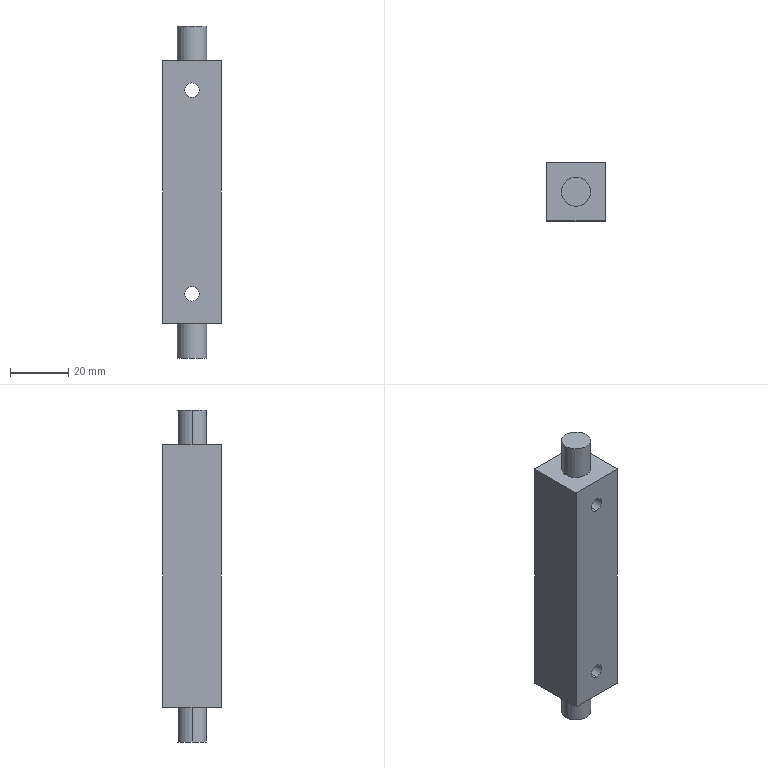Part | STEP file | rotating shaft | 1 solid | 16 faces | box 20 x 20 x 114 mm | volume 37100 mm3 | cylinder 8 | plane 8 | commonest cylinder face diameters 5 x4 10 x4
STEP:
#1=CARTESIAN_POINT('',(0.,-10.,32.5));
#2=VERTEX_POINT('',#1);
#3=CARTESIAN_POINT('',(0.,-10.,37.5));
#4=VERTEX_POINT('',#3);
#5=CARTESIAN_POINT('',(0.,-10.,35.));
#6=DIRECTION('',(0.,1.,0.));
#7=DIRECTION('',(0.,0.,1.));
#8=AXIS2_PLACEMENT_3D('',#5,#6,#7);
#9=CIRCLE('',#8,2.5);
#10=EDGE_CURVE('',#2,#4,#9,.T.);
#11=ORIENTED_EDGE('',*,*,#10,.F.);
#12=CARTESIAN_POINT('',(0.,10.,32.5));
#13=VERTEX_POINT('',#12);
#14=CARTESIAN_POINT('',(0.,10.,32.5));
#15=DIRECTION('',(0.,1.,0.));
#16=VECTOR('',#15,1000.);
#17=LINE('',#14,#16);
#18=EDGE_CURVE('',#2,#13,#17,.T.);
#19=ORIENTED_EDGE('',*,*,#18,.T.);
#20=CARTESIAN_POINT('',(0.,10.,37.5));
#21=VERTEX_POINT('',#20);
#22=CARTESIAN_POINT('',(0.,10.,35.));
#23=DIRECTION('',(0.,1.,0.));
#24=DIRECTION('',(0.,0.,1.));
#25=AXIS2_PLACEMENT_3D('',#22,#23,#24);
#26=CIRCLE('',#25,2.5);
#27=EDGE_CURVE('',#13,#21,#26,.T.);
#28=ORIENTED_EDGE('',*,*,#27,.T.);
#29=CARTESIAN_POINT('',(0.,10.,37.5));
#30=DIRECTION('',(0.,1.,0.));
#31=VECTOR('',#30,1000.);
#32=LINE('',#29,#31);
#33=EDGE_CURVE('',#4,#21,#32,.T.);
#34=ORIENTED_EDGE('',*,*,#33,.F.);
#35=EDGE_LOOP('',(#11,#19,#28,#34));
#36=FACE_OUTER_BOUND('',#35,.T.);
#37=CARTESIAN_POINT('',(0.,10.,35.));
#38=DIRECTION('',(0.,1.,0.));
#39=DIRECTION('',(0.,0.,1.));
#40=AXIS2_PLACEMENT_3D('',#37,#38,#39);
#41=CYLINDRICAL_SURFACE('',#40,2.5);
#42=ADVANCED_FACE('',(#36),#41,.F.);
#43=CARTESIAN_POINT('',(0.,-10.,-37.5));
#44=VERTEX_POINT('',#43);
#45=CARTESIAN_POINT('',(0.,-10.,-32.5));
#46=VERTEX_POINT('',#45);
#47=CARTESIAN_POINT('',(0.,-10.,-35.));
#48=DIRECTION('',(0.,1.,0.));
#49=DIRECTION('',(0.,0.,1.));
#50=AXIS2_PLACEMENT_3D('',#47,#48,#49);
#51=CIRCLE('',#50,2.5);
#52=EDGE_CURVE('',#44,#46,#51,.T.);
#53=ORIENTED_EDGE('',*,*,#52,.F.);
#54=CARTESIAN_POINT('',(0.,10.,-37.5));
#55=VERTEX_POINT('',#54);
#56=CARTESIAN_POINT('',(0.,10.,-37.5));
#57=DIRECTION('',(0.,1.,0.));
#58=VECTOR('',#57,1000.);
#59=LINE('',#56,#58);
#60=EDGE_CURVE('',#44,#55,#59,.T.);
#61=ORIENTED_EDGE('',*,*,#60,.T.);
#62=CARTESIAN_POINT('',(0.,10.,-32.5));
#63=VERTEX_POINT('',#62);
#64=CARTESIAN_POINT('',(0.,10.,-35.));
#65=DIRECTION('',(0.,1.,0.));
#66=DIRECTION('',(0.,0.,1.));
#67=AXIS2_PLACEMENT_3D('',#64,#65,#66);
#68=CIRCLE('',#67,2.5);
#69=EDGE_CURVE('',#55,#63,#68,.T.);
#70=ORIENTED_EDGE('',*,*,#69,.T.);
#71=CARTESIAN_POINT('',(0.,10.,-32.5));
#72=DIRECTION('',(0.,1.,0.));
#73=VECTOR('',#72,1000.);
#74=LINE('',#71,#73);
#75=EDGE_CURVE('',#46,#63,#74,.T.);
#76=ORIENTED_EDGE('',*,*,#75,.F.);
#77=EDGE_LOOP('',(#53,#61,#70,#76));
#78=FACE_OUTER_BOUND('',#77,.T.);
#79=CARTESIAN_POINT('',(0.,10.,-35.));
#80=DIRECTION('',(0.,1.,0.));
#81=DIRECTION('',(0.,0.,1.));
#82=AXIS2_PLACEMENT_3D('',#79,#80,#81);
#83=CYLINDRICAL_SURFACE('',#82,2.5);
#84=ADVANCED_FACE('',(#78),#83,.F.);
#85=CARTESIAN_POINT('',(-5.,0.,-45.));
#86=VERTEX_POINT('',#85);
#87=CARTESIAN_POINT('',(5.,0.,-45.));
#88=VERTEX_POINT('',#87);
#89=CARTESIAN_POINT('',(0.,0.,-45.));
#90=DIRECTION('',(0.,0.,-1.));
#91=DIRECTION('',(-1.,0.,0.));
#92=AXIS2_PLACEMENT_3D('',#89,#90,#91);
#93=CIRCLE('',#92,5.);
#94=EDGE_CURVE('',#86,#88,#93,.T.);
#95=ORIENTED_EDGE('',*,*,#94,.T.);
#96=CARTESIAN_POINT('',(5.,0.,-57.));
#97=VERTEX_POINT('',#96);
#98=CARTESIAN_POINT('',(5.,0.,-45.));
#99=DIRECTION('',(0.,0.,-1.));
#100=VECTOR('',#99,1000.);
#101=LINE('',#98,#100);
#102=EDGE_CURVE('',#88,#97,#101,.T.);
#103=ORIENTED_EDGE('',*,*,#102,.T.);
#104=CARTESIAN_POINT('',(-5.,0.,-57.));
#105=VERTEX_POINT('',#104);
#106=CARTESIAN_POINT('',(0.,0.,-57.));
#107=DIRECTION('',(0.,0.,-1.));
#108=DIRECTION('',(-1.,0.,0.));
#109=AXIS2_PLACEMENT_3D('',#106,#107,#108);
#110=CIRCLE('',#109,5.);
#111=EDGE_CURVE('',#105,#97,#110,.T.);
#112=ORIENTED_EDGE('',*,*,#111,.F.);
#113=CARTESIAN_POINT('',(-5.,0.,-45.));
#114=DIRECTION('',(0.,0.,-1.));
#115=VECTOR('',#114,1000.);
#116=LINE('',#113,#115);
#117=EDGE_CURVE('',#86,#105,#116,.T.);
#118=ORIENTED_EDGE('',*,*,#117,.F.);
#119=EDGE_LOOP('',(#95,#103,#112,#118));
#120=FACE_OUTER_BOUND('',#119,.T.);
#121=CARTESIAN_POINT('',(0.,0.,-45.));
#122=DIRECTION('',(0.,0.,-1.));
#123=DIRECTION('',(-1.,0.,0.));
#124=AXIS2_PLACEMENT_3D('',#121,#122,#123);
#125=CYLINDRICAL_SURFACE('',#124,5.);
#126=ADVANCED_FACE('',(#120),#125,.T.);
#127=CARTESIAN_POINT('',(5.,0.,45.));
#128=VERTEX_POINT('',#127);
#129=CARTESIAN_POINT('',(-5.,0.,45.));
#130=VERTEX_POINT('',#129);
#131=CARTESIAN_POINT('',(0.,0.,45.));
#132=DIRECTION('',(0.,0.,1.));
#133=DIRECTION('',(1.,0.,0.));
#134=AXIS2_PLACEMENT_3D('',#131,#132,#133);
#135=CIRCLE('',#134,5.);
#136=EDGE_CURVE('',#128,#130,#135,.T.);
#137=ORIENTED_EDGE('',*,*,#136,.T.);
#138=CARTESIAN_POINT('',(-5.,0.,57.));
#139=VERTEX_POINT('',#138);
#140=CARTESIAN_POINT('',(-5.,0.,45.));
#141=DIRECTION('',(0.,0.,1.));
#142=VECTOR('',#141,1000.);
#143=LINE('',#140,#142);
#144=EDGE_CURVE('',#130,#139,#143,.T.);
#145=ORIENTED_EDGE('',*,*,#144,.T.);
#146=CARTESIAN_POINT('',(5.,0.,57.));
#147=VERTEX_POINT('',#146);
#148=CARTESIAN_POINT('',(0.,0.,57.));
#149=DIRECTION('',(0.,0.,1.));
#150=DIRECTION('',(1.,0.,0.));
#151=AXIS2_PLACEMENT_3D('',#148,#149,#150);
#152=CIRCLE('',#151,5.);
#153=EDGE_CURVE('',#147,#139,#152,.T.);
#154=ORIENTED_EDGE('',*,*,#153,.F.);
#155=CARTESIAN_POINT('',(5.,0.,45.));
#156=DIRECTION('',(0.,0.,1.));
#157=VECTOR('',#156,1000.);
#158=LINE('',#155,#157);
#159=EDGE_CURVE('',#128,#147,#158,.T.);
#160=ORIENTED_EDGE('',*,*,#159,.F.);
#161=EDGE_LOOP('',(#137,#145,#154,#160));
#162=FACE_OUTER_BOUND('',#161,.T.);
#163=CARTESIAN_POINT('',(0.,0.,45.));
#164=DIRECTION('',(0.,0.,1.));
#165=DIRECTION('',(1.,0.,0.));
#166=AXIS2_PLACEMENT_3D('',#163,#164,#165);
#167=CYLINDRICAL_SURFACE('',#166,5.);
#168=ADVANCED_FACE('',(#162),#167,.T.);
#169=CARTESIAN_POINT('',(10.,10.,-45.));
#170=VERTEX_POINT('',#169);
#171=CARTESIAN_POINT('',(10.,-10.,-45.));
#172=VERTEX_POINT('',#171);
#173=CARTESIAN_POINT('',(10.,10.,-45.));
#174=DIRECTION('',(0.,-1.,0.));
#175=VECTOR('',#174,1000.);
#176=LINE('',#173,#175);
#177=EDGE_CURVE('',#170,#172,#176,.T.);
#178=ORIENTED_EDGE('',*,*,#177,.F.);
#179=CARTESIAN_POINT('',(10.,10.,45.));
#180=VERTEX_POINT('',#179);
#181=CARTESIAN_POINT('',(10.,10.,57.));
#182=DIRECTION('',(0.,0.,-1.));
#183=VECTOR('',#182,1000.);
#184=LINE('',#181,#183);
#185=EDGE_CURVE('',#180,#170,#184,.T.);
#186=ORIENTED_EDGE('',*,*,#185,.F.);
#187=CARTESIAN_POINT('',(10.,-10.,45.));
#188=VERTEX_POINT('',#187);
#189=CARTESIAN_POINT('',(10.,10.,45.));
#190=DIRECTION('',(0.,1.,0.));
#191=VECTOR('',#190,1000.);
#192=LINE('',#189,#191);
#193=EDGE_CURVE('',#188,#180,#192,.T.);
#194=ORIENTED_EDGE('',*,*,#193,.F.);
#195=CARTESIAN_POINT('',(10.,-10.,57.));
#196=DIRECTION('',(0.,0.,-1.));
#197=VECTOR('',#196,1000.);
#198=LINE('',#195,#197);
#199=EDGE_CURVE('',#188,#172,#198,.T.);
#200=ORIENTED_EDGE('',*,*,#199,.T.);
#201=EDGE_LOOP('',(#178,#186,#194,#200));
#202=FACE_OUTER_BOUND('',#201,.T.);
#203=CARTESIAN_POINT('',(10.,10.,57.));
#204=DIRECTION('',(-1.,0.,0.));
#205=DIRECTION('',(0.,0.,1.));
#206=AXIS2_PLACEMENT_3D('',#203,#204,#205);
#207=PLANE('',#206);
#208=ADVANCED_FACE('',(#202),#207,.F.);
#209=CARTESIAN_POINT('',(0.,10.,35.));
#210=DIRECTION('',(0.,1.,0.));
#211=DIRECTION('',(0.,0.,1.));
#212=AXIS2_PLACEMENT_3D('',#209,#210,#211);
#213=CIRCLE('',#212,2.5);
#214=EDGE_CURVE('',#21,#13,#213,.T.);
#215=ORIENTED_EDGE('',*,*,#214,.F.);
#216=ORIENTED_EDGE('',*,*,#27,.F.);
#217=EDGE_LOOP('',(#215,#216));
#218=FACE_BOUND('',#217,.T.);
#219=CARTESIAN_POINT('',(0.,10.,-35.));
#220=DIRECTION('',(0.,1.,0.));
#221=DIRECTION('',(0.,0.,1.));
#222=AXIS2_PLACEMENT_3D('',#219,#220,#221);
#223=CIRCLE('',#222,2.5);
#224=EDGE_CURVE('',#63,#55,#223,.T.);
#225=ORIENTED_EDGE('',*,*,#224,.F.);
#226=ORIENTED_EDGE('',*,*,#69,.F.);
#227=EDGE_LOOP('',(#225,#226));
#228=FACE_BOUND('',#227,.T.);
#229=CARTESIAN_POINT('',(-10.,10.,-45.));
#230=VERTEX_POINT('',#229);
#231=CARTESIAN_POINT('',(-10.,10.,-45.));
#232=DIRECTION('',(1.,0.,0.));
#233=VECTOR('',#232,1000.);
#234=LINE('',#231,#233);
#235=EDGE_CURVE('',#230,#170,#234,.T.);
#236=ORIENTED_EDGE('',*,*,#235,.F.);
#237=CARTESIAN_POINT('',(-10.,10.,45.));
#238=VERTEX_POINT('',#237);
#239=CARTESIAN_POINT('',(-10.,10.,57.));
#240=DIRECTION('',(0.,0.,-1.));
#241=VECTOR('',#240,1000.);
#242=LINE('',#239,#241);
#243=EDGE_CURVE('',#238,#230,#242,.T.);
#244=ORIENTED_EDGE('',*,*,#243,.F.);
#245=CARTESIAN_POINT('',(-10.,10.,45.));
#246=DIRECTION('',(-1.,0.,0.));
#247=VECTOR('',#246,1000.);
#248=LINE('',#245,#247);
#249=EDGE_CURVE('',#180,#238,#248,.T.);
#250=ORIENTED_EDGE('',*,*,#249,.F.);
#251=ORIENTED_EDGE('',*,*,#185,.T.);
#252=EDGE_LOOP('',(#236,#244,#250,#251));
#253=FACE_OUTER_BOUND('',#252,.T.);
#254=CARTESIAN_POINT('',(-10.,10.,57.));
#255=DIRECTION('',(0.,-1.,0.));
#256=DIRECTION('',(0.,0.,-1.));
#257=AXIS2_PLACEMENT_3D('',#254,#255,#256);
#258=PLANE('',#257);
#259=ADVANCED_FACE('',(#218,#228,#253),#258,.F.);
#260=CARTESIAN_POINT('',(-10.,-10.,-45.));
#261=VERTEX_POINT('',#260);
#262=CARTESIAN_POINT('',(-10.,10.,-45.));
#263=DIRECTION('',(0.,1.,0.));
#264=VECTOR('',#263,1000.);
#265=LINE('',#262,#264);
#266=EDGE_CURVE('',#261,#230,#265,.T.);
#267=ORIENTED_EDGE('',*,*,#266,.F.);
#268=CARTESIAN_POINT('',(-10.,-10.,45.));
#269=VERTEX_POINT('',#268);
#270=CARTESIAN_POINT('',(-10.,-10.,57.));
#271=DIRECTION('',(0.,0.,-1.));
#272=VECTOR('',#271,1000.);
#273=LINE('',#270,#272);
#274=EDGE_CURVE('',#269,#261,#273,.T.);
#275=ORIENTED_EDGE('',*,*,#274,.F.);
#276=CARTESIAN_POINT('',(-10.,10.,45.));
#277=DIRECTION('',(0.,-1.,0.));
#278=VECTOR('',#277,1000.);
#279=LINE('',#276,#278);
#280=EDGE_CURVE('',#238,#269,#279,.T.);
#281=ORIENTED_EDGE('',*,*,#280,.F.);
#282=ORIENTED_EDGE('',*,*,#243,.T.);
#283=EDGE_LOOP('',(#267,#275,#281,#282));
#284=FACE_OUTER_BOUND('',#283,.T.);
#285=CARTESIAN_POINT('',(-10.,10.,57.));
#286=DIRECTION('',(1.,0.,0.));
#287=DIRECTION('',(0.,1.,0.));
#288=AXIS2_PLACEMENT_3D('',#285,#286,#287);
#289=PLANE('',#288);
#290=ADVANCED_FACE('',(#284),#289,.F.);
#291=CARTESIAN_POINT('',(0.,-10.,35.));
#292=DIRECTION('',(0.,1.,0.));
#293=DIRECTION('',(0.,0.,1.));
#294=AXIS2_PLACEMENT_3D('',#291,#292,#293);
#295=CIRCLE('',#294,2.5);
#296=EDGE_CURVE('',#4,#2,#295,.T.);
#297=ORIENTED_EDGE('',*,*,#296,.T.);
#298=ORIENTED_EDGE('',*,*,#10,.T.);
#299=EDGE_LOOP('',(#297,#298));
#300=FACE_BOUND('',#299,.T.);
#301=CARTESIAN_POINT('',(0.,-10.,-35.));
#302=DIRECTION('',(0.,1.,0.));
#303=DIRECTION('',(0.,0.,1.));
#304=AXIS2_PLACEMENT_3D('',#301,#302,#303);
#305=CIRCLE('',#304,2.5);
#306=EDGE_CURVE('',#46,#44,#305,.T.);
#307=ORIENTED_EDGE('',*,*,#306,.T.);
#308=ORIENTED_EDGE('',*,*,#52,.T.);
#309=EDGE_LOOP('',(#307,#308));
#310=FACE_BOUND('',#309,.T.);
#311=CARTESIAN_POINT('',(-10.,-10.,-45.));
#312=DIRECTION('',(-1.,0.,0.));
#313=VECTOR('',#312,1000.);
#314=LINE('',#311,#313);
#315=EDGE_CURVE('',#172,#261,#314,.T.);
#316=ORIENTED_EDGE('',*,*,#315,.F.);
#317=ORIENTED_EDGE('',*,*,#199,.F.);
#318=CARTESIAN_POINT('',(-10.,-10.,45.));
#319=DIRECTION('',(1.,0.,0.));
#320=VECTOR('',#319,1000.);
#321=LINE('',#318,#320);
#322=EDGE_CURVE('',#269,#188,#321,.T.);
#323=ORIENTED_EDGE('',*,*,#322,.F.);
#324=ORIENTED_EDGE('',*,*,#274,.T.);
#325=EDGE_LOOP('',(#316,#317,#323,#324));
#326=FACE_OUTER_BOUND('',#325,.T.);
#327=CARTESIAN_POINT('',(-10.,-10.,57.));
#328=DIRECTION('',(0.,1.,0.));
#329=DIRECTION('',(0.,0.,1.));
#330=AXIS2_PLACEMENT_3D('',#327,#328,#329);
#331=PLANE('',#330);
#332=ADVANCED_FACE('',(#300,#310,#326),#331,.F.);
#333=ORIENTED_EDGE('',*,*,#136,.F.);
#334=CARTESIAN_POINT('',(0.,0.,45.));
#335=DIRECTION('',(0.,0.,1.));
#336=DIRECTION('',(1.,0.,0.));
#337=AXIS2_PLACEMENT_3D('',#334,#335,#336);
#338=CIRCLE('',#337,5.);
#339=EDGE_CURVE('',#130,#128,#338,.T.);
#340=ORIENTED_EDGE('',*,*,#339,.F.);
#341=EDGE_LOOP('',(#333,#340));
#342=FACE_BOUND('',#341,.T.);
#343=ORIENTED_EDGE('',*,*,#193,.T.);
#344=ORIENTED_EDGE('',*,*,#249,.T.);
#345=ORIENTED_EDGE('',*,*,#280,.T.);
#346=ORIENTED_EDGE('',*,*,#322,.T.);
#347=EDGE_LOOP('',(#343,#344,#345,#346));
#348=FACE_OUTER_BOUND('',#347,.T.);
#349=CARTESIAN_POINT('',(0.,0.,45.));
#350=DIRECTION('',(0.,0.,1.));
#351=DIRECTION('',(1.,0.,0.));
#352=AXIS2_PLACEMENT_3D('',#349,#350,#351);
#353=PLANE('',#352);
#354=ADVANCED_FACE('',(#342,#348),#353,.T.);
#355=ORIENTED_EDGE('',*,*,#144,.F.);
#356=ORIENTED_EDGE('',*,*,#339,.T.);
#357=ORIENTED_EDGE('',*,*,#159,.T.);
#358=CARTESIAN_POINT('',(0.,0.,57.));
#359=DIRECTION('',(0.,0.,1.));
#360=DIRECTION('',(1.,0.,0.));
#361=AXIS2_PLACEMENT_3D('',#358,#359,#360);
#362=CIRCLE('',#361,5.);
#363=EDGE_CURVE('',#139,#147,#362,.T.);
#364=ORIENTED_EDGE('',*,*,#363,.F.);
#365=EDGE_LOOP('',(#355,#356,#357,#364));
#366=FACE_OUTER_BOUND('',#365,.T.);
#367=CARTESIAN_POINT('',(0.,0.,45.));
#368=DIRECTION('',(0.,0.,1.));
#369=DIRECTION('',(1.,0.,0.));
#370=AXIS2_PLACEMENT_3D('',#367,#368,#369);
#371=CYLINDRICAL_SURFACE('',#370,5.);
#372=ADVANCED_FACE('',(#366),#371,.T.);
#373=ORIENTED_EDGE('',*,*,#153,.T.);
#374=ORIENTED_EDGE('',*,*,#363,.T.);
#375=EDGE_LOOP('',(#373,#374));
#376=FACE_OUTER_BOUND('',#375,.T.);
#377=CARTESIAN_POINT('',(0.,0.,57.));
#378=DIRECTION('',(0.,0.,1.));
#379=DIRECTION('',(1.,0.,0.));
#380=AXIS2_PLACEMENT_3D('',#377,#378,#379);
#381=PLANE('',#380);
#382=ADVANCED_FACE('',(#376),#381,.T.);
#383=ORIENTED_EDGE('',*,*,#94,.F.);
#384=CARTESIAN_POINT('',(0.,0.,-45.));
#385=DIRECTION('',(0.,0.,-1.));
#386=DIRECTION('',(-1.,0.,0.));
#387=AXIS2_PLACEMENT_3D('',#384,#385,#386);
#388=CIRCLE('',#387,5.);
#389=EDGE_CURVE('',#88,#86,#388,.T.);
#390=ORIENTED_EDGE('',*,*,#389,.F.);
#391=EDGE_LOOP('',(#383,#390));
#392=FACE_BOUND('',#391,.T.);
#393=ORIENTED_EDGE('',*,*,#177,.T.);
#394=ORIENTED_EDGE('',*,*,#315,.T.);
#395=ORIENTED_EDGE('',*,*,#266,.T.);
#396=ORIENTED_EDGE('',*,*,#235,.T.);
#397=EDGE_LOOP('',(#393,#394,#395,#396));
#398=FACE_OUTER_BOUND('',#397,.T.);
#399=CARTESIAN_POINT('',(0.,0.,-45.));
#400=DIRECTION('',(0.,0.,-1.));
#401=DIRECTION('',(-1.,0.,0.));
#402=AXIS2_PLACEMENT_3D('',#399,#400,#401);
#403=PLANE('',#402);
#404=ADVANCED_FACE('',(#392,#398),#403,.T.);
#405=ORIENTED_EDGE('',*,*,#102,.F.);
#406=ORIENTED_EDGE('',*,*,#389,.T.);
#407=ORIENTED_EDGE('',*,*,#117,.T.);
#408=CARTESIAN_POINT('',(0.,0.,-57.));
#409=DIRECTION('',(0.,0.,-1.));
#410=DIRECTION('',(-1.,0.,0.));
#411=AXIS2_PLACEMENT_3D('',#408,#409,#410);
#412=CIRCLE('',#411,5.);
#413=EDGE_CURVE('',#97,#105,#412,.T.);
#414=ORIENTED_EDGE('',*,*,#413,.F.);
#415=EDGE_LOOP('',(#405,#406,#407,#414));
#416=FACE_OUTER_BOUND('',#415,.T.);
#417=CARTESIAN_POINT('',(0.,0.,-45.));
#418=DIRECTION('',(0.,0.,-1.));
#419=DIRECTION('',(-1.,0.,0.));
#420=AXIS2_PLACEMENT_3D('',#417,#418,#419);
#421=CYLINDRICAL_SURFACE('',#420,5.);
#422=ADVANCED_FACE('',(#416),#421,.T.);
#423=ORIENTED_EDGE('',*,*,#111,.T.);
#424=ORIENTED_EDGE('',*,*,#413,.T.);
#425=EDGE_LOOP('',(#423,#424));
#426=FACE_OUTER_BOUND('',#425,.T.);
#427=CARTESIAN_POINT('',(0.,0.,-57.));
#428=DIRECTION('',(0.,0.,1.));
#429=DIRECTION('',(1.,0.,0.));
#430=AXIS2_PLACEMENT_3D('',#427,#428,#429);
#431=PLANE('',#430);
#432=ADVANCED_FACE('',(#426),#431,.F.);
#433=ORIENTED_EDGE('',*,*,#60,.F.);
#434=ORIENTED_EDGE('',*,*,#306,.F.);
#435=ORIENTED_EDGE('',*,*,#75,.T.);
#436=ORIENTED_EDGE('',*,*,#224,.T.);
#437=EDGE_LOOP('',(#433,#434,#435,#436));
#438=FACE_OUTER_BOUND('',#437,.T.);
#439=CARTESIAN_POINT('',(0.,10.,-35.));
#440=DIRECTION('',(0.,1.,0.));
#441=DIRECTION('',(0.,0.,1.));
#442=AXIS2_PLACEMENT_3D('',#439,#440,#441);
#443=CYLINDRICAL_SURFACE('',#442,2.5);
#444=ADVANCED_FACE('',(#438),#443,.F.);
#445=ORIENTED_EDGE('',*,*,#18,.F.);
#446=ORIENTED_EDGE('',*,*,#296,.F.);
#447=ORIENTED_EDGE('',*,*,#33,.T.);
#448=ORIENTED_EDGE('',*,*,#214,.T.);
#449=EDGE_LOOP('',(#445,#446,#447,#448));
#450=FACE_OUTER_BOUND('',#449,.T.);
#451=CARTESIAN_POINT('',(0.,10.,35.));
#452=DIRECTION('',(0.,1.,0.));
#453=DIRECTION('',(0.,0.,1.));
#454=AXIS2_PLACEMENT_3D('',#451,#452,#453);
#455=CYLINDRICAL_SURFACE('',#454,2.5);
#456=ADVANCED_FACE('',(#450),#455,.F.);
#457=CLOSED_SHELL('',(#42,#84,#126,#168,#208,#259,#290,#332,#354,#372,#382,#404,#422,#432,#444,#456));
#458=MANIFOLD_SOLID_BREP('',#457);
#459=CARTESIAN_POINT('',(0.,0.,0.));
#460=DIRECTION('',(0.,0.,1.));
#461=DIRECTION('',(1.,0.,0.));
#462=AXIS2_PLACEMENT_3D('',#459,#460,#461);
#463=(LENGTH_UNIT()NAMED_UNIT(*)SI_UNIT(.MILLI.,.METRE.));
#464=UNCERTAINTY_MEASURE_WITH_UNIT(LENGTH_MEASURE(0.00001),#463,'','');
#465=(NAMED_UNIT(*)PLANE_ANGLE_UNIT()SI_UNIT($,.RADIAN.));
#466=(NAMED_UNIT(*)SI_UNIT($,.STERADIAN.)SOLID_ANGLE_UNIT());
#467=(GEOMETRIC_REPRESENTATION_CONTEXT(3)GLOBAL_UNCERTAINTY_ASSIGNED_CONTEXT((#464))GLOBAL_UNIT_ASSIGNED_CONTEXT((#463,#465,#466))REPRESENTATION_CONTEXT('',''));
#468=ADVANCED_BREP_SHAPE_REPRESENTATION('',(#458,#462),#467);